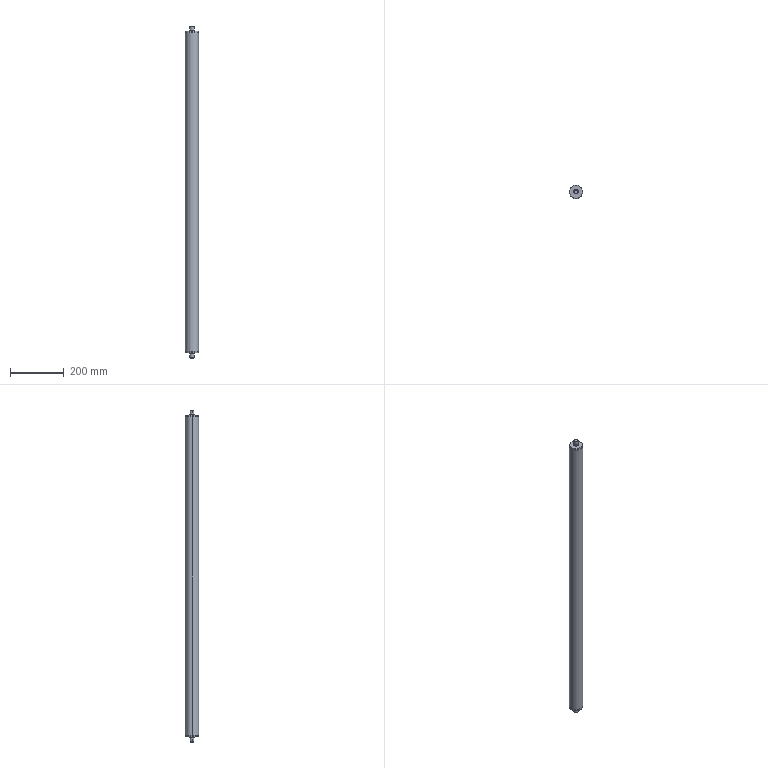Part | SolidWorks | features Chamfer 2, ICE 2, RevCut 1, Revolution 1 | 1 solid | 30 faces | box 50 x 50 x 1240 mm | volume 604574 mm3 | cylinder 14 | cone 8 | plane 8 | commonest cylinder face diameters 15 x6 17 x4 46 x2 50 x2
STEP:
#1=CARTESIAN_POINT('',(6.5,0.,320.));
#2=VERTEX_POINT('',#1);
#3=CARTESIAN_POINT('',(-6.5,0.,320.));
#4=VERTEX_POINT('',#3);
#5=CARTESIAN_POINT('',(0.,0.,320.));
#6=DIRECTION('',(0.,0.,1.));
#7=DIRECTION('',(-1.,0.,0.));
#8=AXIS2_PLACEMENT_3D('',#5,#6,#7);
#9=CIRCLE('',#8,6.5);
#10=EDGE_CURVE('',#2,#4,#9,.T.);
#11=ORIENTED_EDGE('',*,*,#10,.F.);
#12=CARTESIAN_POINT('',(7.5,0.,319.));
#13=VERTEX_POINT('',#12);
#14=CARTESIAN_POINT('',(6.5,0.,320.));
#15=DIRECTION('',(0.7071,0.,-0.7071));
#16=VECTOR('',#15,1000.);
#17=LINE('',#14,#16);
#18=EDGE_CURVE('',#2,#13,#17,.T.);
#19=ORIENTED_EDGE('',*,*,#18,.T.);
#20=CARTESIAN_POINT('',(-7.5,0.,319.));
#21=VERTEX_POINT('',#20);
#22=CARTESIAN_POINT('',(0.,0.,319.));
#23=DIRECTION('',(0.,0.,-1.));
#24=DIRECTION('',(-1.,0.,0.));
#25=AXIS2_PLACEMENT_3D('',#22,#23,#24);
#26=CIRCLE('',#25,7.5);
#27=EDGE_CURVE('',#21,#13,#26,.T.);
#28=ORIENTED_EDGE('',*,*,#27,.F.);
#29=CARTESIAN_POINT('',(-6.5,0.,320.));
#30=DIRECTION('',(-0.7071,0.,-0.7071));
#31=VECTOR('',#30,1000.);
#32=LINE('',#29,#31);
#33=EDGE_CURVE('',#4,#21,#32,.T.);
#34=ORIENTED_EDGE('',*,*,#33,.F.);
#35=EDGE_LOOP('',(#11,#19,#28,#34));
#36=FACE_OUTER_BOUND('',#35,.T.);
#37=CARTESIAN_POINT('',(0.,0.,320.));
#38=DIRECTION('',(0.,0.,-1.));
#39=DIRECTION('',(-1.,0.,0.));
#40=AXIS2_PLACEMENT_3D('',#37,#38,#39);
#41=CONICAL_SURFACE('',#40,6.5,0.7854);
#42=ADVANCED_FACE('',(#36),#41,.T.);
#43=CARTESIAN_POINT('',(-6.5,0.,-920.));
#44=VERTEX_POINT('',#43);
#45=CARTESIAN_POINT('',(6.5,0.,-920.));
#46=VERTEX_POINT('',#45);
#47=CARTESIAN_POINT('',(0.,0.,-920.));
#48=DIRECTION('',(0.,0.,-1.));
#49=DIRECTION('',(1.,0.,0.));
#50=AXIS2_PLACEMENT_3D('',#47,#48,#49);
#51=CIRCLE('',#50,6.5);
#52=EDGE_CURVE('',#44,#46,#51,.T.);
#53=ORIENTED_EDGE('',*,*,#52,.F.);
#54=CARTESIAN_POINT('',(-7.5,0.,-919.));
#55=VERTEX_POINT('',#54);
#56=CARTESIAN_POINT('',(-7.5,0.,-919.));
#57=DIRECTION('',(-0.7071,0.,0.7071));
#58=VECTOR('',#57,1000.);
#59=LINE('',#56,#58);
#60=EDGE_CURVE('',#44,#55,#59,.T.);
#61=ORIENTED_EDGE('',*,*,#60,.T.);
#62=CARTESIAN_POINT('',(7.5,0.,-919.));
#63=VERTEX_POINT('',#62);
#64=CARTESIAN_POINT('',(0.,0.,-919.));
#65=DIRECTION('',(0.,0.,1.));
#66=DIRECTION('',(1.,0.,0.));
#67=AXIS2_PLACEMENT_3D('',#64,#65,#66);
#68=CIRCLE('',#67,7.5);
#69=EDGE_CURVE('',#63,#55,#68,.T.);
#70=ORIENTED_EDGE('',*,*,#69,.F.);
#71=CARTESIAN_POINT('',(7.5,0.,-919.));
#72=DIRECTION('',(0.7071,0.,0.7071));
#73=VECTOR('',#72,1000.);
#74=LINE('',#71,#73);
#75=EDGE_CURVE('',#46,#63,#74,.T.);
#76=ORIENTED_EDGE('',*,*,#75,.F.);
#77=EDGE_LOOP('',(#53,#61,#70,#76));
#78=FACE_OUTER_BOUND('',#77,.T.);
#79=CARTESIAN_POINT('',(0.,0.,-919.));
#80=DIRECTION('',(0.,0.,1.));
#81=DIRECTION('',(1.,0.,0.));
#82=AXIS2_PLACEMENT_3D('',#79,#80,#81);
#83=CONICAL_SURFACE('',#82,7.5,0.7854);
#84=ADVANCED_FACE('',(#78),#83,.T.);
#85=CARTESIAN_POINT('',(24.118,0.,300.));
#86=VERTEX_POINT('',#85);
#87=CARTESIAN_POINT('',(-24.118,0.,300.));
#88=VERTEX_POINT('',#87);
#89=CARTESIAN_POINT('',(0.,0.,300.));
#90=DIRECTION('',(0.,0.,1.));
#91=DIRECTION('',(-1.,0.,0.));
#92=AXIS2_PLACEMENT_3D('',#89,#90,#91);
#93=CIRCLE('',#92,24.118);
#94=EDGE_CURVE('',#86,#88,#93,.T.);
#95=ORIENTED_EDGE('',*,*,#94,.F.);
#96=CARTESIAN_POINT('',(25.,0.,295.));
#97=VERTEX_POINT('',#96);
#98=CARTESIAN_POINT('',(24.118,0.,300.));
#99=DIRECTION('',(0.1736,0.,-0.9848));
#100=VECTOR('',#99,1000.);
#101=LINE('',#98,#100);
#102=EDGE_CURVE('',#86,#97,#101,.T.);
#103=ORIENTED_EDGE('',*,*,#102,.T.);
#104=CARTESIAN_POINT('',(-25.,0.,295.));
#105=VERTEX_POINT('',#104);
#106=CARTESIAN_POINT('',(0.,0.,295.));
#107=DIRECTION('',(0.,0.,-1.));
#108=DIRECTION('',(-1.,0.,0.));
#109=AXIS2_PLACEMENT_3D('',#106,#107,#108);
#110=CIRCLE('',#109,25.);
#111=EDGE_CURVE('',#105,#97,#110,.T.);
#112=ORIENTED_EDGE('',*,*,#111,.F.);
#113=CARTESIAN_POINT('',(-24.118,0.,300.));
#114=DIRECTION('',(-0.1736,0.,-0.9848));
#115=VECTOR('',#114,1000.);
#116=LINE('',#113,#115);
#117=EDGE_CURVE('',#88,#105,#116,.T.);
#118=ORIENTED_EDGE('',*,*,#117,.F.);
#119=EDGE_LOOP('',(#95,#103,#112,#118));
#120=FACE_OUTER_BOUND('',#119,.T.);
#121=CARTESIAN_POINT('',(0.,0.,300.));
#122=DIRECTION('',(0.,0.,-1.));
#123=DIRECTION('',(-1.,0.,0.));
#124=AXIS2_PLACEMENT_3D('',#121,#122,#123);
#125=CONICAL_SURFACE('',#124,24.118,0.1745);
#126=ADVANCED_FACE('',(#120),#125,.T.);
#127=CARTESIAN_POINT('',(-24.118,0.,-900.));
#128=VERTEX_POINT('',#127);
#129=CARTESIAN_POINT('',(24.118,0.,-900.));
#130=VERTEX_POINT('',#129);
#131=CARTESIAN_POINT('',(0.,0.,-900.));
#132=DIRECTION('',(0.,0.,-1.));
#133=DIRECTION('',(1.,0.,0.));
#134=AXIS2_PLACEMENT_3D('',#131,#132,#133);
#135=CIRCLE('',#134,24.118);
#136=EDGE_CURVE('',#128,#130,#135,.T.);
#137=ORIENTED_EDGE('',*,*,#136,.F.);
#138=CARTESIAN_POINT('',(-25.,0.,-895.));
#139=VERTEX_POINT('',#138);
#140=CARTESIAN_POINT('',(-25.,0.,-895.));
#141=DIRECTION('',(-0.1736,0.,0.9848));
#142=VECTOR('',#141,1000.);
#143=LINE('',#140,#142);
#144=EDGE_CURVE('',#128,#139,#143,.T.);
#145=ORIENTED_EDGE('',*,*,#144,.T.);
#146=CARTESIAN_POINT('',(25.,0.,-895.));
#147=VERTEX_POINT('',#146);
#148=CARTESIAN_POINT('',(0.,0.,-895.));
#149=DIRECTION('',(0.,0.,1.));
#150=DIRECTION('',(1.,0.,0.));
#151=AXIS2_PLACEMENT_3D('',#148,#149,#150);
#152=CIRCLE('',#151,25.);
#153=EDGE_CURVE('',#147,#139,#152,.T.);
#154=ORIENTED_EDGE('',*,*,#153,.F.);
#155=CARTESIAN_POINT('',(25.,0.,-895.));
#156=DIRECTION('',(0.1736,0.,0.9848));
#157=VECTOR('',#156,1000.);
#158=LINE('',#155,#157);
#159=EDGE_CURVE('',#130,#147,#158,.T.);
#160=ORIENTED_EDGE('',*,*,#159,.F.);
#161=EDGE_LOOP('',(#137,#145,#154,#160));
#162=FACE_OUTER_BOUND('',#161,.T.);
#163=CARTESIAN_POINT('',(0.,0.,-895.));
#164=DIRECTION('',(0.,0.,1.));
#165=DIRECTION('',(1.,0.,0.));
#166=AXIS2_PLACEMENT_3D('',#163,#164,#165);
#167=CONICAL_SURFACE('',#166,25.,0.1745);
#168=ADVANCED_FACE('',(#162),#167,.T.);
#169=CARTESIAN_POINT('',(8.5,0.,300.));
#170=VERTEX_POINT('',#169);
#171=CARTESIAN_POINT('',(-8.5,0.,300.));
#172=VERTEX_POINT('',#171);
#173=CARTESIAN_POINT('',(0.,0.,300.));
#174=DIRECTION('',(0.,0.,1.));
#175=DIRECTION('',(1.,0.,0.));
#176=AXIS2_PLACEMENT_3D('',#173,#174,#175);
#177=CIRCLE('',#176,8.5);
#178=EDGE_CURVE('',#170,#172,#177,.T.);
#179=ORIENTED_EDGE('',*,*,#178,.T.);
#180=CARTESIAN_POINT('',(-8.5,0.,305.));
#181=VERTEX_POINT('',#180);
#182=CARTESIAN_POINT('',(-8.5,0.,320.));
#183=DIRECTION('',(0.,0.,1.));
#184=VECTOR('',#183,1000.);
#185=LINE('',#182,#184);
#186=EDGE_CURVE('',#172,#181,#185,.T.);
#187=ORIENTED_EDGE('',*,*,#186,.T.);
#188=CARTESIAN_POINT('',(8.5,0.,305.));
#189=VERTEX_POINT('',#188);
#190=CARTESIAN_POINT('',(0.,0.,305.));
#191=DIRECTION('',(0.,0.,1.));
#192=DIRECTION('',(1.,0.,0.));
#193=AXIS2_PLACEMENT_3D('',#190,#191,#192);
#194=CIRCLE('',#193,8.5);
#195=EDGE_CURVE('',#189,#181,#194,.T.);
#196=ORIENTED_EDGE('',*,*,#195,.F.);
#197=CARTESIAN_POINT('',(8.5,0.,320.));
#198=DIRECTION('',(0.,0.,1.));
#199=VECTOR('',#198,1000.);
#200=LINE('',#197,#199);
#201=EDGE_CURVE('',#170,#189,#200,.T.);
#202=ORIENTED_EDGE('',*,*,#201,.F.);
#203=EDGE_LOOP('',(#179,#187,#196,#202));
#204=FACE_OUTER_BOUND('',#203,.T.);
#205=CARTESIAN_POINT('',(0.,0.,320.));
#206=DIRECTION('',(0.,0.,1.));
#207=DIRECTION('',(1.,0.,0.));
#208=AXIS2_PLACEMENT_3D('',#205,#206,#207);
#209=CYLINDRICAL_SURFACE('',#208,8.5);
#210=ADVANCED_FACE('',(#204),#209,.T.);
#211=CARTESIAN_POINT('',(7.5,0.,305.));
#212=VERTEX_POINT('',#211);
#213=CARTESIAN_POINT('',(-7.5,0.,305.));
#214=VERTEX_POINT('',#213);
#215=CARTESIAN_POINT('',(0.,0.,305.));
#216=DIRECTION('',(0.,0.,1.));
#217=DIRECTION('',(1.,0.,0.));
#218=AXIS2_PLACEMENT_3D('',#215,#216,#217);
#219=CIRCLE('',#218,7.5);
#220=EDGE_CURVE('',#212,#214,#219,.T.);
#221=ORIENTED_EDGE('',*,*,#220,.T.);
#222=CARTESIAN_POINT('',(-7.5,0.,320.));
#223=DIRECTION('',(0.,0.,1.));
#224=VECTOR('',#223,1000.);
#225=LINE('',#222,#224);
#226=EDGE_CURVE('',#214,#21,#225,.T.);
#227=ORIENTED_EDGE('',*,*,#226,.T.);
#228=ORIENTED_EDGE('',*,*,#27,.T.);
#229=CARTESIAN_POINT('',(7.5,0.,320.));
#230=DIRECTION('',(0.,0.,1.));
#231=VECTOR('',#230,1000.);
#232=LINE('',#229,#231);
#233=EDGE_CURVE('',#212,#13,#232,.T.);
#234=ORIENTED_EDGE('',*,*,#233,.F.);
#235=EDGE_LOOP('',(#221,#227,#228,#234));
#236=FACE_OUTER_BOUND('',#235,.T.);
#237=CARTESIAN_POINT('',(0.,0.,320.));
#238=DIRECTION('',(0.,0.,1.));
#239=DIRECTION('',(1.,0.,0.));
#240=AXIS2_PLACEMENT_3D('',#237,#238,#239);
#241=CYLINDRICAL_SURFACE('',#240,7.5);
#242=ADVANCED_FACE('',(#236),#241,.T.);
#243=ORIENTED_EDGE('',*,*,#69,.T.);
#244=CARTESIAN_POINT('',(-7.5,0.,-905.));
#245=VERTEX_POINT('',#244);
#246=CARTESIAN_POINT('',(-7.5,0.,320.));
#247=DIRECTION('',(0.,0.,1.));
#248=VECTOR('',#247,1000.);
#249=LINE('',#246,#248);
#250=EDGE_CURVE('',#55,#245,#249,.T.);
#251=ORIENTED_EDGE('',*,*,#250,.T.);
#252=CARTESIAN_POINT('',(7.5,0.,-905.));
#253=VERTEX_POINT('',#252);
#254=CARTESIAN_POINT('',(0.,0.,-905.));
#255=DIRECTION('',(0.,0.,1.));
#256=DIRECTION('',(1.,0.,0.));
#257=AXIS2_PLACEMENT_3D('',#254,#255,#256);
#258=CIRCLE('',#257,7.5);
#259=EDGE_CURVE('',#253,#245,#258,.T.);
#260=ORIENTED_EDGE('',*,*,#259,.F.);
#261=CARTESIAN_POINT('',(7.5,0.,320.));
#262=DIRECTION('',(0.,0.,1.));
#263=VECTOR('',#262,1000.);
#264=LINE('',#261,#263);
#265=EDGE_CURVE('',#63,#253,#264,.T.);
#266=ORIENTED_EDGE('',*,*,#265,.F.);
#267=EDGE_LOOP('',(#243,#251,#260,#266));
#268=FACE_OUTER_BOUND('',#267,.T.);
#269=CARTESIAN_POINT('',(0.,0.,320.));
#270=DIRECTION('',(0.,0.,1.));
#271=DIRECTION('',(1.,0.,0.));
#272=AXIS2_PLACEMENT_3D('',#269,#270,#271);
#273=CYLINDRICAL_SURFACE('',#272,7.5);
#274=ADVANCED_FACE('',(#268),#273,.T.);
#275=CARTESIAN_POINT('',(8.5,0.,-905.));
#276=VERTEX_POINT('',#275);
#277=CARTESIAN_POINT('',(-8.5,0.,-905.));
#278=VERTEX_POINT('',#277);
#279=CARTESIAN_POINT('',(0.,0.,-905.));
#280=DIRECTION('',(0.,0.,1.));
#281=DIRECTION('',(1.,0.,0.));
#282=AXIS2_PLACEMENT_3D('',#279,#280,#281);
#283=CIRCLE('',#282,8.5);
#284=EDGE_CURVE('',#276,#278,#283,.T.);
#285=ORIENTED_EDGE('',*,*,#284,.T.);
#286=CARTESIAN_POINT('',(-8.5,0.,-900.));
#287=VERTEX_POINT('',#286);
#288=CARTESIAN_POINT('',(-8.5,0.,320.));
#289=DIRECTION('',(0.,0.,1.));
#290=VECTOR('',#289,1000.);
#291=LINE('',#288,#290);
#292=EDGE_CURVE('',#278,#287,#291,.T.);
#293=ORIENTED_EDGE('',*,*,#292,.T.);
#294=CARTESIAN_POINT('',(8.5,0.,-900.));
#295=VERTEX_POINT('',#294);
#296=CARTESIAN_POINT('',(0.,0.,-900.));
#297=DIRECTION('',(0.,0.,1.));
#298=DIRECTION('',(1.,0.,0.));
#299=AXIS2_PLACEMENT_3D('',#296,#297,#298);
#300=CIRCLE('',#299,8.5);
#301=EDGE_CURVE('',#295,#287,#300,.T.);
#302=ORIENTED_EDGE('',*,*,#301,.F.);
#303=CARTESIAN_POINT('',(8.5,0.,320.));
#304=DIRECTION('',(0.,0.,1.));
#305=VECTOR('',#304,1000.);
#306=LINE('',#303,#305);
#307=EDGE_CURVE('',#276,#295,#306,.T.);
#308=ORIENTED_EDGE('',*,*,#307,.F.);
#309=EDGE_LOOP('',(#285,#293,#302,#308));
#310=FACE_OUTER_BOUND('',#309,.T.);
#311=CARTESIAN_POINT('',(0.,0.,320.));
#312=DIRECTION('',(0.,0.,1.));
#313=DIRECTION('',(1.,0.,0.));
#314=AXIS2_PLACEMENT_3D('',#311,#312,#313);
#315=CYLINDRICAL_SURFACE('',#314,8.5);
#316=ADVANCED_FACE('',(#310),#315,.T.);
#317=ORIENTED_EDGE('',*,*,#153,.T.);
#318=CARTESIAN_POINT('',(-25.,0.,320.));
#319=DIRECTION('',(0.,0.,1.));
#320=VECTOR('',#319,1000.);
#321=LINE('',#318,#320);
#322=EDGE_CURVE('',#139,#105,#321,.T.);
#323=ORIENTED_EDGE('',*,*,#322,.T.);
#324=ORIENTED_EDGE('',*,*,#111,.T.);
#325=CARTESIAN_POINT('',(25.,0.,320.));
#326=DIRECTION('',(0.,0.,1.));
#327=VECTOR('',#326,1000.);
#328=LINE('',#325,#327);
#329=EDGE_CURVE('',#147,#97,#328,.T.);
#330=ORIENTED_EDGE('',*,*,#329,.F.);
#331=EDGE_LOOP('',(#317,#323,#324,#330));
#332=FACE_OUTER_BOUND('',#331,.T.);
#333=CARTESIAN_POINT('',(0.,0.,320.));
#334=DIRECTION('',(0.,0.,1.));
#335=DIRECTION('',(1.,0.,0.));
#336=AXIS2_PLACEMENT_3D('',#333,#334,#335);
#337=CYLINDRICAL_SURFACE('',#336,25.);
#338=ADVANCED_FACE('',(#332),#337,.T.);
#339=CARTESIAN_POINT('',(0.,0.,300.));
#340=DIRECTION('',(0.,0.,1.));
#341=DIRECTION('',(-1.,0.,0.));
#342=AXIS2_PLACEMENT_3D('',#339,#340,#341);
#343=CIRCLE('',#342,24.118);
#344=EDGE_CURVE('',#88,#86,#343,.T.);
#345=ORIENTED_EDGE('',*,*,#344,.T.);
#346=ORIENTED_EDGE('',*,*,#94,.T.);
#347=EDGE_LOOP('',(#345,#346));
#348=FACE_OUTER_BOUND('',#347,.T.);
#349=ORIENTED_EDGE('',*,*,#178,.F.);
#350=CARTESIAN_POINT('',(0.,0.,300.));
#351=DIRECTION('',(0.,0.,1.));
#352=DIRECTION('',(1.,0.,0.));
#353=AXIS2_PLACEMENT_3D('',#350,#351,#352);
#354=CIRCLE('',#353,8.5);
#355=EDGE_CURVE('',#172,#170,#354,.T.);
#356=ORIENTED_EDGE('',*,*,#355,.F.);
#357=EDGE_LOOP('',(#349,#356));
#358=FACE_BOUND('',#357,.T.);
#359=CARTESIAN_POINT('',(0.,8.5,300.));
#360=DIRECTION('',(0.,0.,-1.));
#361=DIRECTION('',(-1.,0.,0.));
#362=AXIS2_PLACEMENT_3D('',#359,#360,#361);
#363=PLANE('',#362);
#364=ADVANCED_FACE('',(#348,#358),#363,.F.);
#365=ORIENTED_EDGE('',*,*,#322,.F.);
#366=CARTESIAN_POINT('',(0.,0.,-895.));
#367=DIRECTION('',(0.,0.,1.));
#368=DIRECTION('',(1.,0.,0.));
#369=AXIS2_PLACEMENT_3D('',#366,#367,#368);
#370=CIRCLE('',#369,25.);
#371=EDGE_CURVE('',#139,#147,#370,.T.);
#372=ORIENTED_EDGE('',*,*,#371,.T.);
#373=ORIENTED_EDGE('',*,*,#329,.T.);
#374=CARTESIAN_POINT('',(0.,0.,295.));
#375=DIRECTION('',(0.,0.,-1.));
#376=DIRECTION('',(-1.,0.,0.));
#377=AXIS2_PLACEMENT_3D('',#374,#375,#376);
#378=CIRCLE('',#377,25.);
#379=EDGE_CURVE('',#97,#105,#378,.T.);
#380=ORIENTED_EDGE('',*,*,#379,.T.);
#381=EDGE_LOOP('',(#365,#372,#373,#380));
#382=FACE_OUTER_BOUND('',#381,.T.);
#383=CARTESIAN_POINT('',(0.,0.,320.));
#384=DIRECTION('',(0.,0.,1.));
#385=DIRECTION('',(1.,0.,0.));
#386=AXIS2_PLACEMENT_3D('',#383,#384,#385);
#387=CYLINDRICAL_SURFACE('',#386,25.);
#388=ADVANCED_FACE('',(#382),#387,.T.);
#389=CARTESIAN_POINT('',(0.,0.,-900.));
#390=DIRECTION('',(0.,0.,-1.));
#391=DIRECTION('',(1.,0.,0.));
#392=AXIS2_PLACEMENT_3D('',#389,#390,#391);
#393=CIRCLE('',#392,24.118);
#394=EDGE_CURVE('',#130,#128,#393,.T.);
#395=ORIENTED_EDGE('',*,*,#394,.T.);
#396=ORIENTED_EDGE('',*,*,#136,.T.);
#397=EDGE_LOOP('',(#395,#396));
#398=FACE_OUTER_BOUND('',#397,.T.);
#399=ORIENTED_EDGE('',*,*,#301,.T.);
#400=CARTESIAN_POINT('',(0.,0.,-900.));
#401=DIRECTION('',(0.,0.,1.));
#402=DIRECTION('',(1.,0.,0.));
#403=AXIS2_PLACEMENT_3D('',#400,#401,#402);
#404=CIRCLE('',#403,8.5);
#405=EDGE_CURVE('',#287,#295,#404,.T.);
#406=ORIENTED_EDGE('',*,*,#405,.T.);
#407=EDGE_LOOP('',(#399,#406));
#408=FACE_BOUND('',#407,.T.);
#409=CARTESIAN_POINT('',(0.,8.5,-900.));
#410=DIRECTION('',(0.,0.,1.));
#411=DIRECTION('',(1.,0.,0.));
#412=AXIS2_PLACEMENT_3D('',#409,#410,#411);
#413=PLANE('',#412);
#414=ADVANCED_FACE('',(#398,#408),#413,.F.);
#415=ORIENTED_EDGE('',*,*,#292,.F.);
#416=CARTESIAN_POINT('',(0.,0.,-905.));
#417=DIRECTION('',(0.,0.,1.));
#418=DIRECTION('',(1.,0.,0.));
#419=AXIS2_PLACEMENT_3D('',#416,#417,#418);
#420=CIRCLE('',#419,8.5);
#421=EDGE_CURVE('',#278,#276,#420,.T.);
#422=ORIENTED_EDGE('',*,*,#421,.T.);
#423=ORIENTED_EDGE('',*,*,#307,.T.);
#424=ORIENTED_EDGE('',*,*,#405,.F.);
#425=EDGE_LOOP('',(#415,#422,#423,#424));
#426=FACE_OUTER_BOUND('',#425,.T.);
#427=CARTESIAN_POINT('',(0.,0.,320.));
#428=DIRECTION('',(0.,0.,1.));
#429=DIRECTION('',(1.,0.,0.));
#430=AXIS2_PLACEMENT_3D('',#427,#428,#429);
#431=CYLINDRICAL_SURFACE('',#430,8.5);
#432=ADVANCED_FACE('',(#426),#431,.T.);
#433=ORIENTED_EDGE('',*,*,#284,.F.);
#434=ORIENTED_EDGE('',*,*,#421,.F.);
#435=EDGE_LOOP('',(#433,#434));
#436=FACE_OUTER_BOUND('',#435,.T.);
#437=ORIENTED_EDGE('',*,*,#259,.T.);
#438=CARTESIAN_POINT('',(0.,0.,-905.));
#439=DIRECTION('',(0.,0.,1.));
#440=DIRECTION('',(1.,0.,0.));
#441=AXIS2_PLACEMENT_3D('',#438,#439,#440);
#442=CIRCLE('',#441,7.5);
#443=EDGE_CURVE('',#245,#253,#442,.T.);
#444=ORIENTED_EDGE('',*,*,#443,.T.);
#445=EDGE_LOOP('',(#437,#444));
#446=FACE_BOUND('',#445,.T.);
#447=CARTESIAN_POINT('',(0.,7.5,-905.));
#448=DIRECTION('',(0.,0.,1.));
#449=DIRECTION('',(1.,0.,0.));
#450=AXIS2_PLACEMENT_3D('',#447,#448,#449);
#451=PLANE('',#450);
#452=ADVANCED_FACE('',(#436,#446),#451,.F.);
#453=ORIENTED_EDGE('',*,*,#250,.F.);
#454=CARTESIAN_POINT('',(0.,0.,-919.));
#455=DIRECTION('',(0.,0.,1.));
#456=DIRECTION('',(1.,0.,0.));
#457=AXIS2_PLACEMENT_3D('',#454,#455,#456);
#458=CIRCLE('',#457,7.5);
#459=EDGE_CURVE('',#55,#63,#458,.T.);
#460=ORIENTED_EDGE('',*,*,#459,.T.);
#461=ORIENTED_EDGE('',*,*,#265,.T.);
#462=ORIENTED_EDGE('',*,*,#443,.F.);
#463=EDGE_LOOP('',(#453,#460,#461,#462));
#464=FACE_OUTER_BOUND('',#463,.T.);
#465=CARTESIAN_POINT('',(0.,0.,320.));
#466=DIRECTION('',(0.,0.,1.));
#467=DIRECTION('',(1.,0.,0.));
#468=AXIS2_PLACEMENT_3D('',#465,#466,#467);
#469=CYLINDRICAL_SURFACE('',#468,7.5);
#470=ADVANCED_FACE('',(#464),#469,.T.);
#471=CARTESIAN_POINT('',(0.,0.,-920.));
#472=DIRECTION('',(0.,0.,-1.));
#473=DIRECTION('',(1.,0.,0.));
#474=AXIS2_PLACEMENT_3D('',#471,#472,#473);
#475=CIRCLE('',#474,6.5);
#476=EDGE_CURVE('',#46,#44,#475,.T.);
#477=ORIENTED_EDGE('',*,*,#476,.T.);
#478=ORIENTED_EDGE('',*,*,#52,.T.);
#479=EDGE_LOOP('',(#477,#478));
#480=FACE_OUTER_BOUND('',#479,.T.);
#481=CARTESIAN_POINT('',(0.,0.,-920.));
#482=DIRECTION('',(0.,0.,1.));
#483=DIRECTION('',(1.,0.,0.));
#484=AXIS2_PLACEMENT_3D('',#481,#482,#483);
#485=PLANE('',#484);
#486=ADVANCED_FACE('',(#480),#485,.F.);
#487=CARTESIAN_POINT('',(0.,0.,320.));
#488=DIRECTION('',(0.,0.,1.));
#489=DIRECTION('',(-1.,0.,0.));
#490=AXIS2_PLACEMENT_3D('',#487,#488,#489);
#491=CIRCLE('',#490,6.5);
#492=EDGE_CURVE('',#4,#2,#491,.T.);
#493=ORIENTED_EDGE('',*,*,#492,.T.);
#494=ORIENTED_EDGE('',*,*,#10,.T.);
#495=EDGE_LOOP('',(#493,#494));
#496=FACE_OUTER_BOUND('',#495,.T.);
#497=CARTESIAN_POINT('',(0.,0.,320.));
#498=DIRECTION('',(0.,0.,-1.));
#499=DIRECTION('',(-1.,0.,0.));
#500=AXIS2_PLACEMENT_3D('',#497,#498,#499);
#501=PLANE('',#500);
#502=ADVANCED_FACE('',(#496),#501,.F.);
#503=ORIENTED_EDGE('',*,*,#226,.F.);
#504=CARTESIAN_POINT('',(0.,0.,305.));
#505=DIRECTION('',(0.,0.,1.));
#506=DIRECTION('',(1.,0.,0.));
#507=AXIS2_PLACEMENT_3D('',#504,#505,#506);
#508=CIRCLE('',#507,7.5);
#509=EDGE_CURVE('',#214,#212,#508,.T.);
#510=ORIENTED_EDGE('',*,*,#509,.T.);
#511=ORIENTED_EDGE('',*,*,#233,.T.);
#512=CARTESIAN_POINT('',(0.,0.,319.));
#513=DIRECTION('',(0.,0.,-1.));
#514=DIRECTION('',(-1.,0.,0.));
#515=AXIS2_PLACEMENT_3D('',#512,#513,#514);
#516=CIRCLE('',#515,7.5);
#517=EDGE_CURVE('',#13,#21,#516,.T.);
#518=ORIENTED_EDGE('',*,*,#517,.T.);
#519=EDGE_LOOP('',(#503,#510,#511,#518));
#520=FACE_OUTER_BOUND('',#519,.T.);
#521=CARTESIAN_POINT('',(0.,0.,320.));
#522=DIRECTION('',(0.,0.,1.));
#523=DIRECTION('',(1.,0.,0.));
#524=AXIS2_PLACEMENT_3D('',#521,#522,#523);
#525=CYLINDRICAL_SURFACE('',#524,7.5);
#526=ADVANCED_FACE('',(#520),#525,.T.);
#527=ORIENTED_EDGE('',*,*,#220,.F.);
#528=ORIENTED_EDGE('',*,*,#509,.F.);
#529=EDGE_LOOP('',(#527,#528));
#530=FACE_BOUND('',#529,.T.);
#531=ORIENTED_EDGE('',*,*,#195,.T.);
#532=CARTESIAN_POINT('',(0.,0.,305.));
#533=DIRECTION('',(0.,0.,1.));
#534=DIRECTION('',(1.,0.,0.));
#535=AXIS2_PLACEMENT_3D('',#532,#533,#534);
#536=CIRCLE('',#535,8.5);
#537=EDGE_CURVE('',#181,#189,#536,.T.);
#538=ORIENTED_EDGE('',*,*,#537,.T.);
#539=EDGE_LOOP('',(#531,#538));
#540=FACE_OUTER_BOUND('',#539,.T.);
#541=CARTESIAN_POINT('',(0.,7.5,305.));
#542=DIRECTION('',(0.,0.,-1.));
#543=DIRECTION('',(-1.,0.,0.));
#544=AXIS2_PLACEMENT_3D('',#541,#542,#543);
#545=PLANE('',#544);
#546=ADVANCED_FACE('',(#530,#540),#545,.F.);
#547=ORIENTED_EDGE('',*,*,#186,.F.);
#548=ORIENTED_EDGE('',*,*,#355,.T.);
#549=ORIENTED_EDGE('',*,*,#201,.T.);
#550=ORIENTED_EDGE('',*,*,#537,.F.);
#551=EDGE_LOOP('',(#547,#548,#549,#550));
#552=FACE_OUTER_BOUND('',#551,.T.);
#553=CARTESIAN_POINT('',(0.,0.,320.));
#554=DIRECTION('',(0.,0.,1.));
#555=DIRECTION('',(1.,0.,0.));
#556=AXIS2_PLACEMENT_3D('',#553,#554,#555);
#557=CYLINDRICAL_SURFACE('',#556,8.5);
#558=ADVANCED_FACE('',(#552),#557,.T.);
#559=ORIENTED_EDGE('',*,*,#144,.F.);
#560=ORIENTED_EDGE('',*,*,#394,.F.);
#561=ORIENTED_EDGE('',*,*,#159,.T.);
#562=ORIENTED_EDGE('',*,*,#371,.F.);
#563=EDGE_LOOP('',(#559,#560,#561,#562));
#564=FACE_OUTER_BOUND('',#563,.T.);
#565=CARTESIAN_POINT('',(0.,0.,-895.));
#566=DIRECTION('',(0.,0.,1.));
#567=DIRECTION('',(1.,0.,0.));
#568=AXIS2_PLACEMENT_3D('',#565,#566,#567);
#569=CONICAL_SURFACE('',#568,25.,0.1745);
#570=ADVANCED_FACE('',(#564),#569,.T.);
#571=ORIENTED_EDGE('',*,*,#102,.F.);
#572=ORIENTED_EDGE('',*,*,#344,.F.);
#573=ORIENTED_EDGE('',*,*,#117,.T.);
#574=ORIENTED_EDGE('',*,*,#379,.F.);
#575=EDGE_LOOP('',(#571,#572,#573,#574));
#576=FACE_OUTER_BOUND('',#575,.T.);
#577=CARTESIAN_POINT('',(0.,0.,300.));
#578=DIRECTION('',(0.,0.,-1.));
#579=DIRECTION('',(-1.,0.,0.));
#580=AXIS2_PLACEMENT_3D('',#577,#578,#579);
#581=CONICAL_SURFACE('',#580,24.118,0.1745);
#582=ADVANCED_FACE('',(#576),#581,.T.);
#583=ORIENTED_EDGE('',*,*,#60,.F.);
#584=ORIENTED_EDGE('',*,*,#476,.F.);
#585=ORIENTED_EDGE('',*,*,#75,.T.);
#586=ORIENTED_EDGE('',*,*,#459,.F.);
#587=EDGE_LOOP('',(#583,#584,#585,#586));
#588=FACE_OUTER_BOUND('',#587,.T.);
#589=CARTESIAN_POINT('',(0.,0.,-919.));
#590=DIRECTION('',(0.,0.,1.));
#591=DIRECTION('',(1.,0.,0.));
#592=AXIS2_PLACEMENT_3D('',#589,#590,#591);
#593=CONICAL_SURFACE('',#592,7.5,0.7854);
#594=ADVANCED_FACE('',(#588),#593,.T.);
#595=ORIENTED_EDGE('',*,*,#18,.F.);
#596=ORIENTED_EDGE('',*,*,#492,.F.);
#597=ORIENTED_EDGE('',*,*,#33,.T.);
#598=ORIENTED_EDGE('',*,*,#517,.F.);
#599=EDGE_LOOP('',(#595,#596,#597,#598));
#600=FACE_OUTER_BOUND('',#599,.T.);
#601=CARTESIAN_POINT('',(0.,0.,320.));
#602=DIRECTION('',(0.,0.,-1.));
#603=DIRECTION('',(-1.,0.,0.));
#604=AXIS2_PLACEMENT_3D('',#601,#602,#603);
#605=CONICAL_SURFACE('',#604,6.5,0.7854);
#606=ADVANCED_FACE('',(#600),#605,.T.);
#607=CLOSED_SHELL('',(#42,#84,#126,#168,#210,#242,#274,#316,#338,#364,#388,#414,#432,#452,#470,#486,#502,#526,#546,#558,#570,#582,#594,#606));
#608=CARTESIAN_POINT('',(23.,0.,292.));
#609=VERTEX_POINT('',#608);
#610=CARTESIAN_POINT('',(-23.,0.,292.));
#611=VERTEX_POINT('',#610);
#612=CARTESIAN_POINT('',(0.,0.,292.));
#613=DIRECTION('',(0.,0.,-1.));
#614=DIRECTION('',(-1.,0.,0.));
#615=AXIS2_PLACEMENT_3D('',#612,#613,#614);
#616=CIRCLE('',#615,23.);
#617=EDGE_CURVE('',#609,#611,#616,.T.);
#618=ORIENTED_EDGE('',*,*,#617,.F.);
#619=CARTESIAN_POINT('',(23.,0.,-892.));
#620=VERTEX_POINT('',#619);
#621=CARTESIAN_POINT('',(23.,0.,-920.));
#622=DIRECTION('',(0.,0.,-1.));
#623=VECTOR('',#622,1000.);
#624=LINE('',#621,#623);
#625=EDGE_CURVE('',#609,#620,#624,.T.);
#626=ORIENTED_EDGE('',*,*,#625,.T.);
#627=CARTESIAN_POINT('',(-23.,0.,-892.));
#628=VERTEX_POINT('',#627);
#629=CARTESIAN_POINT('',(0.,0.,-892.));
#630=DIRECTION('',(0.,0.,-1.));
#631=DIRECTION('',(-1.,0.,0.));
#632=AXIS2_PLACEMENT_3D('',#629,#630,#631);
#633=CIRCLE('',#632,23.);
#634=EDGE_CURVE('',#620,#628,#633,.T.);
#635=ORIENTED_EDGE('',*,*,#634,.T.);
#636=CARTESIAN_POINT('',(-23.,0.,-920.));
#637=DIRECTION('',(0.,0.,-1.));
#638=VECTOR('',#637,1000.);
#639=LINE('',#636,#638);
#640=EDGE_CURVE('',#611,#628,#639,.T.);
#641=ORIENTED_EDGE('',*,*,#640,.F.);
#642=EDGE_LOOP('',(#618,#626,#635,#641));
#643=FACE_OUTER_BOUND('',#642,.T.);
#644=CARTESIAN_POINT('',(0.,0.,-920.));
#645=DIRECTION('',(0.,0.,-1.));
#646=DIRECTION('',(-1.,0.,0.));
#647=AXIS2_PLACEMENT_3D('',#644,#645,#646);
#648=CYLINDRICAL_SURFACE('',#647,23.);
#649=ADVANCED_FACE('',(#643),#648,.F.);
#650=CARTESIAN_POINT('',(-7.5,0.,292.));
#651=VERTEX_POINT('',#650);
#652=CARTESIAN_POINT('',(7.5,0.,292.));
#653=VERTEX_POINT('',#652);
#654=CARTESIAN_POINT('',(0.,0.,292.));
#655=DIRECTION('',(0.,0.,-1.));
#656=DIRECTION('',(-1.,0.,0.));
#657=AXIS2_PLACEMENT_3D('',#654,#655,#656);
#658=CIRCLE('',#657,7.5);
#659=EDGE_CURVE('',#651,#653,#658,.T.);
#660=ORIENTED_EDGE('',*,*,#659,.T.);
#661=CARTESIAN_POINT('',(7.5,0.,-892.));
#662=VERTEX_POINT('',#661);
#663=CARTESIAN_POINT('',(7.5,0.,-920.));
#664=DIRECTION('',(0.,0.,-1.));
#665=VECTOR('',#664,1000.);
#666=LINE('',#663,#665);
#667=EDGE_CURVE('',#653,#662,#666,.T.);
#668=ORIENTED_EDGE('',*,*,#667,.T.);
#669=CARTESIAN_POINT('',(-7.5,0.,-892.));
#670=VERTEX_POINT('',#669);
#671=CARTESIAN_POINT('',(0.,0.,-892.));
#672=DIRECTION('',(0.,0.,-1.));
#673=DIRECTION('',(-1.,0.,0.));
#674=AXIS2_PLACEMENT_3D('',#671,#672,#673);
#675=CIRCLE('',#674,7.5);
#676=EDGE_CURVE('',#670,#662,#675,.T.);
#677=ORIENTED_EDGE('',*,*,#676,.F.);
#678=CARTESIAN_POINT('',(-7.5,0.,-920.));
#679=DIRECTION('',(0.,0.,-1.));
#680=VECTOR('',#679,1000.);
#681=LINE('',#678,#680);
#682=EDGE_CURVE('',#651,#670,#681,.T.);
#683=ORIENTED_EDGE('',*,*,#682,.F.);
#684=EDGE_LOOP('',(#660,#668,#677,#683));
#685=FACE_OUTER_BOUND('',#684,.T.);
#686=CARTESIAN_POINT('',(0.,0.,-920.));
#687=DIRECTION('',(0.,0.,-1.));
#688=DIRECTION('',(-1.,0.,0.));
#689=AXIS2_PLACEMENT_3D('',#686,#687,#688);
#690=CYLINDRICAL_SURFACE('',#689,7.5);
#691=ADVANCED_FACE('',(#685),#690,.T.);
#692=ORIENTED_EDGE('',*,*,#667,.F.);
#693=CARTESIAN_POINT('',(0.,0.,292.));
#694=DIRECTION('',(0.,0.,-1.));
#695=DIRECTION('',(-1.,0.,0.));
#696=AXIS2_PLACEMENT_3D('',#693,#694,#695);
#697=CIRCLE('',#696,7.5);
#698=EDGE_CURVE('',#653,#651,#697,.T.);
#699=ORIENTED_EDGE('',*,*,#698,.T.);
#700=ORIENTED_EDGE('',*,*,#682,.T.);
#701=CARTESIAN_POINT('',(0.,0.,-892.));
#702=DIRECTION('',(0.,0.,-1.));
#703=DIRECTION('',(-1.,0.,0.));
#704=AXIS2_PLACEMENT_3D('',#701,#702,#703);
#705=CIRCLE('',#704,7.5);
#706=EDGE_CURVE('',#662,#670,#705,.T.);
#707=ORIENTED_EDGE('',*,*,#706,.F.);
#708=EDGE_LOOP('',(#692,#699,#700,#707));
#709=FACE_OUTER_BOUND('',#708,.T.);
#710=CARTESIAN_POINT('',(0.,0.,-920.));
#711=DIRECTION('',(0.,0.,-1.));
#712=DIRECTION('',(-1.,0.,0.));
#713=AXIS2_PLACEMENT_3D('',#710,#711,#712);
#714=CYLINDRICAL_SURFACE('',#713,7.5);
#715=ADVANCED_FACE('',(#709),#714,.T.);
#716=ORIENTED_EDGE('',*,*,#676,.T.);
#717=ORIENTED_EDGE('',*,*,#706,.T.);
#718=EDGE_LOOP('',(#716,#717));
#719=FACE_BOUND('',#718,.T.);
#720=CARTESIAN_POINT('',(0.,0.,-892.));
#721=DIRECTION('',(0.,0.,-1.));
#722=DIRECTION('',(-1.,0.,0.));
#723=AXIS2_PLACEMENT_3D('',#720,#721,#722);
#724=CIRCLE('',#723,23.);
#725=EDGE_CURVE('',#628,#620,#724,.T.);
#726=ORIENTED_EDGE('',*,*,#725,.F.);
#727=ORIENTED_EDGE('',*,*,#634,.F.);
#728=EDGE_LOOP('',(#726,#727));
#729=FACE_OUTER_BOUND('',#728,.T.);
#730=CARTESIAN_POINT('',(7.5,0.,-892.));
#731=DIRECTION('',(0.,0.,1.));
#732=DIRECTION('',(1.,0.,0.));
#733=AXIS2_PLACEMENT_3D('',#730,#731,#732);
#734=PLANE('',#733);
#735=ADVANCED_FACE('',(#719,#729),#734,.T.);
#736=ORIENTED_EDGE('',*,*,#625,.F.);
#737=CARTESIAN_POINT('',(0.,0.,292.));
#738=DIRECTION('',(0.,0.,-1.));
#739=DIRECTION('',(-1.,0.,0.));
#740=AXIS2_PLACEMENT_3D('',#737,#738,#739);
#741=CIRCLE('',#740,23.);
#742=EDGE_CURVE('',#611,#609,#741,.T.);
#743=ORIENTED_EDGE('',*,*,#742,.F.);
#744=ORIENTED_EDGE('',*,*,#640,.T.);
#745=ORIENTED_EDGE('',*,*,#725,.T.);
#746=EDGE_LOOP('',(#736,#743,#744,#745));
#747=FACE_OUTER_BOUND('',#746,.T.);
#748=CARTESIAN_POINT('',(0.,0.,-920.));
#749=DIRECTION('',(0.,0.,-1.));
#750=DIRECTION('',(-1.,0.,0.));
#751=AXIS2_PLACEMENT_3D('',#748,#749,#750);
#752=CYLINDRICAL_SURFACE('',#751,23.);
#753=ADVANCED_FACE('',(#747),#752,.F.);
#754=ORIENTED_EDGE('',*,*,#742,.T.);
#755=ORIENTED_EDGE('',*,*,#617,.T.);
#756=EDGE_LOOP('',(#754,#755));
#757=FACE_OUTER_BOUND('',#756,.T.);
#758=ORIENTED_EDGE('',*,*,#659,.F.);
#759=ORIENTED_EDGE('',*,*,#698,.F.);
#760=EDGE_LOOP('',(#758,#759));
#761=FACE_BOUND('',#760,.T.);
#762=CARTESIAN_POINT('',(23.,0.,292.));
#763=DIRECTION('',(0.,0.,-1.));
#764=DIRECTION('',(-1.,0.,0.));
#765=AXIS2_PLACEMENT_3D('',#762,#763,#764);
#766=PLANE('',#765);
#767=ADVANCED_FACE('',(#757,#761),#766,.T.);
#768=CLOSED_SHELL('',(#649,#691,#715,#735,#753,#767));
#769=ORIENTED_CLOSED_SHELL('',*,#768,.F.);
#770=BREP_WITH_VOIDS('',#607,(#769));
#771=CARTESIAN_POINT('',(0.,0.,0.));
#772=DIRECTION('',(0.,0.,1.));
#773=DIRECTION('',(1.,0.,0.));
#774=AXIS2_PLACEMENT_3D('',#771,#772,#773);
#775=(LENGTH_UNIT()NAMED_UNIT(*)SI_UNIT(.MILLI.,.METRE.));
#776=UNCERTAINTY_MEASURE_WITH_UNIT(LENGTH_MEASURE(0.00001),#775,'','');
#777=(NAMED_UNIT(*)PLANE_ANGLE_UNIT()SI_UNIT($,.RADIAN.));
#778=(NAMED_UNIT(*)SI_UNIT($,.STERADIAN.)SOLID_ANGLE_UNIT());
#779=(GEOMETRIC_REPRESENTATION_CONTEXT(3)GLOBAL_UNCERTAINTY_ASSIGNED_CONTEXT((#776))GLOBAL_UNIT_ASSIGNED_CONTEXT((#775,#777,#778))REPRESENTATION_CONTEXT('',''));
#780=ADVANCED_BREP_SHAPE_REPRESENTATION('',(#770,#774),#779);